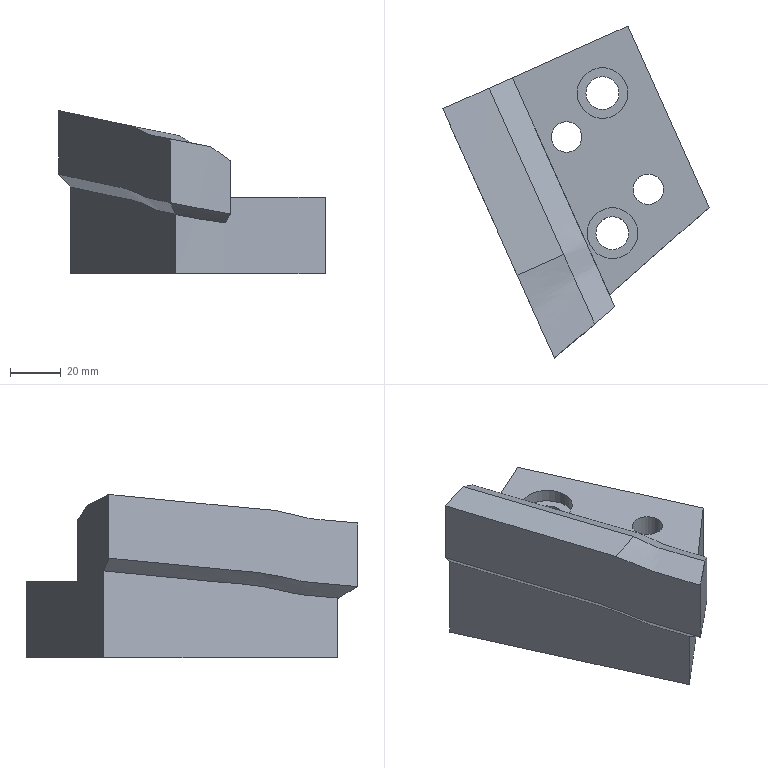Part | NX | features solid 2 | 1 solid | 23 faces | box 104.998 x 130.856 x 64.255 mm | volume 265696 mm3 | plane 9 | spline 8 | cylinder 6 | commonest cylinder face diameters 12 x2 13 x2 20 x2